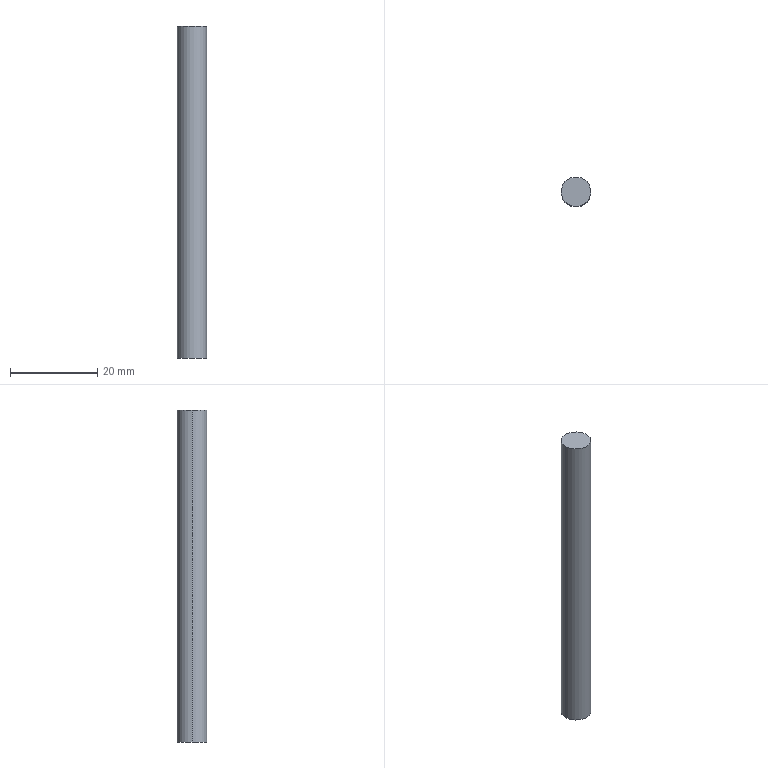Part | SolidWorks | features Extrusion 1 | 1 solid | 4 faces | box 6.756 x 6.756 x 76.2 mm | volume 2732 mm3 | cylinder 2 | plane 2 | commonest cylinder face diameters 6.756 x2
STEP:
#1=CARTESIAN_POINT('',(3.378,0.,38.1));
#2=VERTEX_POINT('',#1);
#3=CARTESIAN_POINT('',(-3.378,0.,38.1));
#4=VERTEX_POINT('',#3);
#5=CARTESIAN_POINT('',(0.,0.,38.1));
#6=DIRECTION('',(0.,0.,1.));
#7=DIRECTION('',(1.,0.,0.));
#8=AXIS2_PLACEMENT_3D('',#5,#6,#7);
#9=CIRCLE('',#8,3.378);
#10=EDGE_CURVE('',#2,#4,#9,.T.);
#11=ORIENTED_EDGE('',*,*,#10,.F.);
#12=CARTESIAN_POINT('',(3.378,0.,-38.1));
#13=VERTEX_POINT('',#12);
#14=CARTESIAN_POINT('',(3.378,0.,38.1));
#15=DIRECTION('',(0.,0.,-1.));
#16=VECTOR('',#15,1000.);
#17=LINE('',#14,#16);
#18=EDGE_CURVE('',#2,#13,#17,.T.);
#19=ORIENTED_EDGE('',*,*,#18,.T.);
#20=CARTESIAN_POINT('',(-3.378,0.,-38.1));
#21=VERTEX_POINT('',#20);
#22=CARTESIAN_POINT('',(0.,0.,-38.1));
#23=DIRECTION('',(0.,0.,1.));
#24=DIRECTION('',(1.,0.,0.));
#25=AXIS2_PLACEMENT_3D('',#22,#23,#24);
#26=CIRCLE('',#25,3.378);
#27=EDGE_CURVE('',#13,#21,#26,.T.);
#28=ORIENTED_EDGE('',*,*,#27,.T.);
#29=CARTESIAN_POINT('',(-3.378,0.,38.1));
#30=DIRECTION('',(0.,0.,-1.));
#31=VECTOR('',#30,1000.);
#32=LINE('',#29,#31);
#33=EDGE_CURVE('',#4,#21,#32,.T.);
#34=ORIENTED_EDGE('',*,*,#33,.F.);
#35=EDGE_LOOP('',(#11,#19,#28,#34));
#36=FACE_OUTER_BOUND('',#35,.T.);
#37=CARTESIAN_POINT('',(0.,0.,38.1));
#38=DIRECTION('',(0.,0.,-1.));
#39=DIRECTION('',(-1.,0.,0.));
#40=AXIS2_PLACEMENT_3D('',#37,#38,#39);
#41=CYLINDRICAL_SURFACE('',#40,3.378);
#42=ADVANCED_FACE('',(#36),#41,.T.);
#43=ORIENTED_EDGE('',*,*,#18,.F.);
#44=CARTESIAN_POINT('',(0.,0.,38.1));
#45=DIRECTION('',(0.,0.,1.));
#46=DIRECTION('',(1.,0.,0.));
#47=AXIS2_PLACEMENT_3D('',#44,#45,#46);
#48=CIRCLE('',#47,3.378);
#49=EDGE_CURVE('',#4,#2,#48,.T.);
#50=ORIENTED_EDGE('',*,*,#49,.F.);
#51=ORIENTED_EDGE('',*,*,#33,.T.);
#52=CARTESIAN_POINT('',(0.,0.,-38.1));
#53=DIRECTION('',(0.,0.,1.));
#54=DIRECTION('',(1.,0.,0.));
#55=AXIS2_PLACEMENT_3D('',#52,#53,#54);
#56=CIRCLE('',#55,3.378);
#57=EDGE_CURVE('',#21,#13,#56,.T.);
#58=ORIENTED_EDGE('',*,*,#57,.T.);
#59=EDGE_LOOP('',(#43,#50,#51,#58));
#60=FACE_OUTER_BOUND('',#59,.T.);
#61=CARTESIAN_POINT('',(0.,0.,38.1));
#62=DIRECTION('',(0.,0.,-1.));
#63=DIRECTION('',(-1.,0.,0.));
#64=AXIS2_PLACEMENT_3D('',#61,#62,#63);
#65=CYLINDRICAL_SURFACE('',#64,3.378);
#66=ADVANCED_FACE('',(#60),#65,.T.);
#67=ORIENTED_EDGE('',*,*,#49,.T.);
#68=ORIENTED_EDGE('',*,*,#10,.T.);
#69=EDGE_LOOP('',(#67,#68));
#70=FACE_OUTER_BOUND('',#69,.T.);
#71=CARTESIAN_POINT('',(0.,0.,38.1));
#72=DIRECTION('',(0.,0.,1.));
#73=DIRECTION('',(1.,0.,0.));
#74=AXIS2_PLACEMENT_3D('',#71,#72,#73);
#75=PLANE('',#74);
#76=ADVANCED_FACE('',(#70),#75,.T.);
#77=ORIENTED_EDGE('',*,*,#57,.F.);
#78=ORIENTED_EDGE('',*,*,#27,.F.);
#79=EDGE_LOOP('',(#77,#78));
#80=FACE_OUTER_BOUND('',#79,.T.);
#81=CARTESIAN_POINT('',(0.,0.,-38.1));
#82=DIRECTION('',(0.,0.,1.));
#83=DIRECTION('',(1.,0.,0.));
#84=AXIS2_PLACEMENT_3D('',#81,#82,#83);
#85=PLANE('',#84);
#86=ADVANCED_FACE('',(#80),#85,.F.);
#87=CLOSED_SHELL('',(#42,#66,#76,#86));
#88=MANIFOLD_SOLID_BREP('',#87);
#89=CARTESIAN_POINT('',(0.,0.,0.));
#90=DIRECTION('',(0.,0.,1.));
#91=DIRECTION('',(1.,0.,0.));
#92=AXIS2_PLACEMENT_3D('',#89,#90,#91);
#93=(LENGTH_UNIT()NAMED_UNIT(*)SI_UNIT(.MILLI.,.METRE.));
#94=UNCERTAINTY_MEASURE_WITH_UNIT(LENGTH_MEASURE(0.00001),#93,'','');
#95=(NAMED_UNIT(*)PLANE_ANGLE_UNIT()SI_UNIT($,.RADIAN.));
#96=(NAMED_UNIT(*)SI_UNIT($,.STERADIAN.)SOLID_ANGLE_UNIT());
#97=(GEOMETRIC_REPRESENTATION_CONTEXT(3)GLOBAL_UNCERTAINTY_ASSIGNED_CONTEXT((#94))GLOBAL_UNIT_ASSIGNED_CONTEXT((#93,#95,#96))REPRESENTATION_CONTEXT('',''));
#98=ADVANCED_BREP_SHAPE_REPRESENTATION('',(#88,#92),#97);